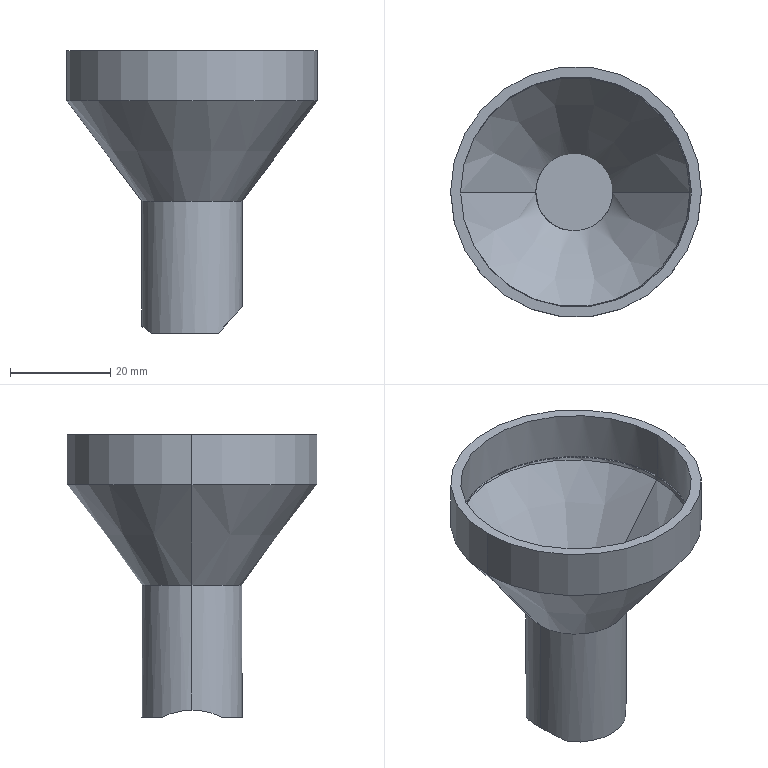Part | SolidWorks | features ICE 2, Blend 1, Cut 1, Extrusion 1, RefAxis 1, RevCut 1, SweepCut 1 | 1 solid | 21 faces | box 50 x 50 x 56.352 mm | volume 10137 mm3 | cylinder 8 | cone 6 | plane 5 | spline 2 | commonest cylinder face diameters 16 x2 20 x2 46 x2 50 x2
STEP:
#1=CARTESIAN_POINT('',(22.69,0.,-10.684));
#2=VERTEX_POINT('',#1);
#3=CARTESIAN_POINT('',(-23.,0.,-10.));
#4=VERTEX_POINT('',#3);
#5=CARTESIAN_POINT('',(-0.1549,0.,-10.342));
#6=DIRECTION('',(0.01498,0.,0.9999));
#7=DIRECTION('',(0.9999,0.,-0.01498));
#8=AXIS2_PLACEMENT_3D('',#5,#6,#7);
#9=CIRCLE('',#8,22.848);
#10=EDGE_CURVE('',#2,#4,#9,.T.);
#11=ORIENTED_EDGE('',*,*,#10,.F.);
#12=CARTESIAN_POINT('',(22.711,0.,-10.));
#13=VERTEX_POINT('',#12);
#14=CARTESIAN_POINT('',(22.69,0.,-10.684));
#15=DIRECTION('',(0.02995,0.,0.9996));
#16=VECTOR('',#15,1000.);
#17=LINE('',#14,#16);
#18=EDGE_CURVE('',#2,#13,#17,.T.);
#19=ORIENTED_EDGE('',*,*,#18,.T.);
#20=CARTESIAN_POINT('',(-23.,0.,-10.));
#21=CARTESIAN_POINT('',(-23.,45.706,-10.));
#22=CARTESIAN_POINT('',(22.711,45.706,-10.));
#23=CARTESIAN_POINT('',(22.711,0.,-10.));
#24=(BOUNDED_CURVE()B_SPLINE_CURVE(3,(#20,#21,#22,#23),.UNSPECIFIED.,.F.,.T.)B_SPLINE_CURVE_WITH_KNOTS((4,4),(3.142,6.283),.UNSPECIFIED.)CURVE()GEOMETRIC_REPRESENTATION_ITEM()RATIONAL_B_SPLINE_CURVE((1.,0.3333,0.3333,1.))REPRESENTATION_ITEM(''));
#25=EDGE_CURVE('',#4,#13,#24,.T.);
#26=ORIENTED_EDGE('',*,*,#25,.F.);
#27=EDGE_LOOP('',(#11,#19,#26));
#28=FACE_OUTER_BOUND('',#27,.T.);
#29=CARTESIAN_POINT('',(-0.1549,0.,-10.342));
#30=DIRECTION('',(0.01498,0.,0.9999));
#31=DIRECTION('',(0.9999,0.,-0.01498));
#32=AXIS2_PLACEMENT_3D('',#29,#30,#31);
#33=CONICAL_SURFACE('',#32,22.848,0.01498);
#34=ADVANCED_FACE('',(#28),#33,.F.);
#35=CARTESIAN_POINT('',(-8.,0.,-30.));
#36=VERTEX_POINT('',#35);
#37=CARTESIAN_POINT('',(7.278,0.,-30.));
#38=VERTEX_POINT('',#37);
#39=CARTESIAN_POINT('',(-8.,0.,-30.));
#40=CARTESIAN_POINT('',(-8.,-15.276,-30.));
#41=CARTESIAN_POINT('',(7.278,-15.276,-30.));
#42=CARTESIAN_POINT('',(7.278,0.,-30.));
#43=(BOUNDED_CURVE()B_SPLINE_CURVE(3,(#39,#40,#41,#42),.UNSPECIFIED.,.F.,.F.)B_SPLINE_CURVE_WITH_KNOTS((4,4),(3.142,6.283),.UNSPECIFIED.)CURVE()GEOMETRIC_REPRESENTATION_ITEM()RATIONAL_B_SPLINE_CURVE((1.,0.3333,0.3333,1.))REPRESENTATION_ITEM(''));
#44=EDGE_CURVE('',#36,#38,#43,.T.);
#45=ORIENTED_EDGE('',*,*,#44,.F.);
#46=CARTESIAN_POINT('',(-8.,0.,-30.));
#47=DIRECTION('',(-0.6,0.,0.8));
#48=VECTOR('',#47,1000.);
#49=LINE('',#46,#48);
#50=EDGE_CURVE('',#36,#4,#49,.T.);
#51=ORIENTED_EDGE('',*,*,#50,.T.);
#52=CARTESIAN_POINT('',(-0.1549,0.,-10.342));
#53=DIRECTION('',(0.01498,0.,0.9999));
#54=DIRECTION('',(0.9999,0.,-0.01498));
#55=AXIS2_PLACEMENT_3D('',#52,#53,#54);
#56=CIRCLE('',#55,22.848);
#57=EDGE_CURVE('',#4,#2,#56,.T.);
#58=ORIENTED_EDGE('',*,*,#57,.T.);
#59=CARTESIAN_POINT('',(7.098,0.,-30.226));
#60=DIRECTION('',(0.6237,0.,0.7817));
#61=VECTOR('',#60,1000.);
#62=LINE('',#59,#61);
#63=EDGE_CURVE('',#38,#2,#62,.T.);
#64=ORIENTED_EDGE('',*,*,#63,.F.);
#65=EDGE_LOOP('',(#45,#51,#58,#64));
#66=FACE_OUTER_BOUND('',#65,.T.);
#67=CARTESIAN_POINT('',(-0.4511,0.,-30.113));
#68=DIRECTION('',(0.01498,0.,0.9999));
#69=DIRECTION('',(0.9999,0.,-0.01498));
#70=AXIS2_PLACEMENT_3D('',#67,#68,#69);
#71=CONICAL_SURFACE('',#70,7.55,0.6585);
#72=ADVANCED_FACE('',(#66),#71,.F.);
#73=CARTESIAN_POINT('',(-8.,0.,-54.334));
#74=VERTEX_POINT('',#73);
#75=CARTESIAN_POINT('',(-3.42,-7.232,-56.352));
#76=VERTEX_POINT('',#75);
#77=CARTESIAN_POINT('',(-8.,0.,-54.334));
#78=CARTESIAN_POINT('',(-8.,-0.3871,-54.334));
#79=CARTESIAN_POINT('',(-7.971,-0.779,-54.35));
#80=CARTESIAN_POINT('',(-7.86,-1.541,-54.411));
#81=CARTESIAN_POINT('',(-7.777,-1.915,-54.456));
#82=CARTESIAN_POINT('',(-7.559,-2.648,-54.575));
#83=CARTESIAN_POINT('',(-7.422,-3.009,-54.648));
#84=CARTESIAN_POINT('',(-7.106,-3.695,-54.816));
#85=CARTESIAN_POINT('',(-6.925,-4.023,-54.91));
#86=CARTESIAN_POINT('',(-6.52,-4.65,-55.114));
#87=CARTESIAN_POINT('',(-6.295,-4.951,-55.226));
#88=CARTESIAN_POINT('',(-5.811,-5.511,-55.455));
#89=CARTESIAN_POINT('',(-5.552,-5.771,-55.573));
#90=CARTESIAN_POINT('',(-5.,-6.256,-55.81));
#91=CARTESIAN_POINT('',(-4.704,-6.481,-55.929));
#92=CARTESIAN_POINT('',(-4.082,-6.89,-56.154));
#93=CARTESIAN_POINT('',(-3.758,-7.072,-56.26));
#94=CARTESIAN_POINT('',(-3.42,-7.232,-56.352));
#95=B_SPLINE_CURVE_WITH_KNOTS('',3,(#77,#78,#79,#80,#81,#82,#83,#84,#85,#86,#87,#88,#89,#90,#91,#92,#93,#94),.UNSPECIFIED.,.F.,.F.,(4,2,2,2,2,2,2,2,4),(0.02654,0.02769,0.02885,0.03,0.03116,0.03231,0.03347,0.03462,0.03578),.UNSPECIFIED.);
#96=EDGE_CURVE('',#74,#76,#95,.T.);
#97=ORIENTED_EDGE('',*,*,#96,.F.);
#98=CARTESIAN_POINT('',(-8.,0.,-40.));
#99=DIRECTION('',(0.,0.,1.));
#100=VECTOR('',#99,1000.);
#101=LINE('',#98,#100);
#102=EDGE_CURVE('',#74,#36,#101,.T.);
#103=ORIENTED_EDGE('',*,*,#102,.T.);
#104=CARTESIAN_POINT('',(8.,0.,-30.));
#105=VERTEX_POINT('',#104);
#106=CARTESIAN_POINT('',(0.,0.,-30.));
#107=DIRECTION('',(0.,0.,1.));
#108=DIRECTION('',(-1.,0.,0.));
#109=AXIS2_PLACEMENT_3D('',#106,#107,#108);
#110=CIRCLE('',#109,8.);
#111=EDGE_CURVE('',#36,#105,#110,.T.);
#112=ORIENTED_EDGE('',*,*,#111,.T.);
#113=CARTESIAN_POINT('',(8.,0.,-51.21));
#114=VERTEX_POINT('',#113);
#115=CARTESIAN_POINT('',(8.,0.,-40.));
#116=DIRECTION('',(0.,0.,1.));
#117=VECTOR('',#116,1000.);
#118=LINE('',#115,#117);
#119=EDGE_CURVE('',#114,#105,#118,.T.);
#120=ORIENTED_EDGE('',*,*,#119,.F.);
#121=CARTESIAN_POINT('',(0.6884,-7.97,-56.352));
#122=VERTEX_POINT('',#121);
#123=CARTESIAN_POINT('',(0.6884,-7.97,-56.352));
#124=CARTESIAN_POINT('',(0.9487,-7.948,-56.271));
#125=CARTESIAN_POINT('',(1.206,-7.913,-56.175));
#126=CARTESIAN_POINT('',(1.702,-7.821,-55.964));
#127=CARTESIAN_POINT('',(1.942,-7.765,-55.848));
#128=CARTESIAN_POINT('',(2.408,-7.633,-55.603));
#129=CARTESIAN_POINT('',(2.635,-7.557,-55.473));
#130=CARTESIAN_POINT('',(3.079,-7.388,-55.203));
#131=CARTESIAN_POINT('',(3.296,-7.293,-55.063));
#132=CARTESIAN_POINT('',(3.926,-6.986,-54.637));
#133=CARTESIAN_POINT('',(4.318,-6.75,-54.347));
#134=CARTESIAN_POINT('',(5.061,-6.212,-53.771));
#135=CARTESIAN_POINT('',(5.412,-5.911,-53.486));
#136=CARTESIAN_POINT('',(6.072,-5.231,-52.932));
#137=CARTESIAN_POINT('',(6.374,-4.859,-52.671));
#138=CARTESIAN_POINT('',(6.781,-4.251,-52.312));
#139=CARTESIAN_POINT('',(6.909,-4.04,-52.199));
#140=CARTESIAN_POINT('',(7.15,-3.598,-51.984));
#141=CARTESIAN_POINT('',(7.262,-3.366,-51.883));
#142=CARTESIAN_POINT('',(7.564,-2.655,-51.61));
#143=CARTESIAN_POINT('',(7.723,-2.156,-51.465));
#144=CARTESIAN_POINT('',(7.888,-1.362,-51.313));
#145=CARTESIAN_POINT('',(7.93,-1.092,-51.275));
#146=CARTESIAN_POINT('',(7.986,-0.5495,-51.223));
#147=CARTESIAN_POINT('',(8.,-0.276,-51.21));
#148=CARTESIAN_POINT('',(8.,0.,-51.21));
#149=B_SPLINE_CURVE_WITH_KNOTS('',3,(#123,#124,#125,#126,#127,#128,#129,#130,#131,#132,#133,#134,#135,#136,#137,#138,#139,#140,#141,#142,#143,#144,#145,#146,#147,#148),.UNSPECIFIED.,.F.,.F.,(4,2,2,2,2,2,2,2,2,2,2,2,4),(0.04003,0.04084,0.04166,0.04247,0.04328,0.04491,0.04654,0.04817,0.04898,0.04979,0.05142,0.05224,0.05305),.UNSPECIFIED.);
#150=EDGE_CURVE('',#122,#114,#149,.T.);
#151=ORIENTED_EDGE('',*,*,#150,.F.);
#152=CARTESIAN_POINT('',(0.,0.,-56.352));
#153=DIRECTION('',(0.,0.,1.));
#154=DIRECTION('',(1.,0.,0.));
#155=AXIS2_PLACEMENT_3D('',#152,#153,#154);
#156=CIRCLE('',#155,8.);
#157=EDGE_CURVE('',#76,#122,#156,.T.);
#158=ORIENTED_EDGE('',*,*,#157,.F.);
#159=EDGE_LOOP('',(#97,#103,#112,#120,#151,#158));
#160=FACE_OUTER_BOUND('',#159,.T.);
#161=CARTESIAN_POINT('',(0.,0.,-40.));
#162=DIRECTION('',(0.,0.,1.));
#163=DIRECTION('',(1.,0.,0.));
#164=AXIS2_PLACEMENT_3D('',#161,#162,#163);
#165=CYLINDRICAL_SURFACE('',#164,8.);
#166=ADVANCED_FACE('',(#160),#165,.F.);
#167=CARTESIAN_POINT('',(-8.076,5.897,-56.352));
#168=VERTEX_POINT('',#167);
#169=CARTESIAN_POINT('',(-10.,0.,-54.908));
#170=VERTEX_POINT('',#169);
#171=CARTESIAN_POINT('',(-8.076,5.897,-56.352));
#172=CARTESIAN_POINT('',(-8.369,5.496,-56.131));
#173=CARTESIAN_POINT('',(-8.635,5.069,-55.93));
#174=CARTESIAN_POINT('',(-9.109,4.158,-55.574));
#175=CARTESIAN_POINT('',(-9.317,3.671,-55.418));
#176=CARTESIAN_POINT('',(-9.651,2.671,-55.168));
#177=CARTESIAN_POINT('',(-9.78,2.154,-55.072));
#178=CARTESIAN_POINT('',(-9.912,1.351,-54.973));
#179=CARTESIAN_POINT('',(-9.945,1.079,-54.949));
#180=CARTESIAN_POINT('',(-9.989,0.5395,-54.916));
#181=CARTESIAN_POINT('',(-10.,0.2697,-54.908));
#182=CARTESIAN_POINT('',(-10.,0.,-54.908));
#183=B_SPLINE_CURVE_WITH_KNOTS('',3,(#171,#172,#173,#174,#175,#176,#177,#178,#179,#180,#181,#182),.UNSPECIFIED.,.F.,.F.,(4,2,2,2,2,4),(0.01131,0.01294,0.01457,0.01619,0.01701,0.01782),.UNSPECIFIED.);
#184=EDGE_CURVE('',#168,#170,#183,.T.);
#185=ORIENTED_EDGE('',*,*,#184,.T.);
#186=CARTESIAN_POINT('',(-10.,0.,-30.));
#187=VERTEX_POINT('',#186);
#188=CARTESIAN_POINT('',(-10.,0.,-40.));
#189=DIRECTION('',(0.,0.,1.));
#190=VECTOR('',#189,1000.);
#191=LINE('',#188,#190);
#192=EDGE_CURVE('',#170,#187,#191,.T.);
#193=ORIENTED_EDGE('',*,*,#192,.T.);
#194=CARTESIAN_POINT('',(10.,0.,-30.));
#195=VERTEX_POINT('',#194);
#196=CARTESIAN_POINT('',(0.,0.,-30.));
#197=DIRECTION('',(0.,0.,-1.));
#198=DIRECTION('',(-1.,0.,0.));
#199=AXIS2_PLACEMENT_3D('',#196,#197,#198);
#200=CIRCLE('',#199,10.);
#201=EDGE_CURVE('',#187,#195,#200,.T.);
#202=ORIENTED_EDGE('',*,*,#201,.T.);
#203=CARTESIAN_POINT('',(10.,0.,-50.997));
#204=VERTEX_POINT('',#203);
#205=CARTESIAN_POINT('',(10.,0.,-40.));
#206=DIRECTION('',(0.,0.,1.));
#207=VECTOR('',#206,1000.);
#208=LINE('',#205,#207);
#209=EDGE_CURVE('',#204,#195,#208,.T.);
#210=ORIENTED_EDGE('',*,*,#209,.F.);
#211=CARTESIAN_POINT('',(5.262,8.504,-56.352));
#212=VERTEX_POINT('',#211);
#213=CARTESIAN_POINT('',(10.,0.,-50.997));
#214=CARTESIAN_POINT('',(10.,0.4979,-50.997));
#215=CARTESIAN_POINT('',(9.963,0.9852,-51.037));
#216=CARTESIAN_POINT('',(9.857,1.702,-51.154));
#217=CARTESIAN_POINT('',(9.813,1.938,-51.203));
#218=CARTESIAN_POINT('',(9.709,2.406,-51.318));
#219=CARTESIAN_POINT('',(9.648,2.639,-51.385));
#220=CARTESIAN_POINT('',(9.446,3.316,-51.609));
#221=CARTESIAN_POINT('',(9.284,3.743,-51.788));
#222=CARTESIAN_POINT('',(8.913,4.556,-52.201));
#223=CARTESIAN_POINT('',(8.703,4.943,-52.435));
#224=CARTESIAN_POINT('',(8.031,6.018,-53.187));
#225=CARTESIAN_POINT('',(7.524,6.631,-53.758));
#226=CARTESIAN_POINT('',(6.426,7.7,-55.009));
#227=CARTESIAN_POINT('',(5.852,8.138,-55.667));
#228=CARTESIAN_POINT('',(5.262,8.504,-56.352));
#229=B_SPLINE_CURVE_WITH_KNOTS('',3,(#213,#214,#215,#216,#217,#218,#219,#220,#221,#222,#223,#224,#225,#226,#227,#228),.UNSPECIFIED.,.F.,.F.,(4,2,2,2,2,2,2,4),(0.01995,0.0214,0.02213,0.02286,0.02431,0.02577,0.02868,0.03159),.UNSPECIFIED.);
#230=EDGE_CURVE('',#204,#212,#229,.T.);
#231=ORIENTED_EDGE('',*,*,#230,.T.);
#232=CARTESIAN_POINT('',(0.,0.,-56.352));
#233=DIRECTION('',(0.,0.,1.));
#234=DIRECTION('',(1.,0.,0.));
#235=AXIS2_PLACEMENT_3D('',#232,#233,#234);
#236=CIRCLE('',#235,10.);
#237=EDGE_CURVE('',#212,#168,#236,.T.);
#238=ORIENTED_EDGE('',*,*,#237,.T.);
#239=EDGE_LOOP('',(#185,#193,#202,#210,#231,#238));
#240=FACE_OUTER_BOUND('',#239,.T.);
#241=CARTESIAN_POINT('',(0.,0.,-40.));
#242=DIRECTION('',(0.,0.,1.));
#243=DIRECTION('',(1.,0.,0.));
#244=AXIS2_PLACEMENT_3D('',#241,#242,#243);
#245=CYLINDRICAL_SURFACE('',#244,10.);
#246=ADVANCED_FACE('',(#240),#245,.T.);
#247=ORIENTED_EDGE('',*,*,#201,.F.);
#248=CARTESIAN_POINT('',(-25.,0.,-10.));
#249=VERTEX_POINT('',#248);
#250=CARTESIAN_POINT('',(-10.,0.,-30.));
#251=DIRECTION('',(-0.6,0.,0.8));
#252=VECTOR('',#251,1000.);
#253=LINE('',#250,#252);
#254=EDGE_CURVE('',#187,#249,#253,.T.);
#255=ORIENTED_EDGE('',*,*,#254,.T.);
#256=CARTESIAN_POINT('',(25.,0.,-10.));
#257=VERTEX_POINT('',#256);
#258=CARTESIAN_POINT('',(0.,0.,-10.));
#259=DIRECTION('',(0.,0.,1.));
#260=DIRECTION('',(1.,0.,0.));
#261=AXIS2_PLACEMENT_3D('',#258,#259,#260);
#262=CIRCLE('',#261,25.);
#263=EDGE_CURVE('',#257,#249,#262,.T.);
#264=ORIENTED_EDGE('',*,*,#263,.F.);
#265=CARTESIAN_POINT('',(10.,0.,-30.));
#266=DIRECTION('',(0.6,0.,0.8));
#267=VECTOR('',#266,1000.);
#268=LINE('',#265,#267);
#269=EDGE_CURVE('',#195,#257,#268,.T.);
#270=ORIENTED_EDGE('',*,*,#269,.F.);
#271=EDGE_LOOP('',(#247,#255,#264,#270));
#272=FACE_OUTER_BOUND('',#271,.T.);
#273=CARTESIAN_POINT('',(0.,0.,-30.));
#274=DIRECTION('',(0.,0.,1.));
#275=DIRECTION('',(1.,0.,0.));
#276=AXIS2_PLACEMENT_3D('',#273,#274,#275);
#277=CONICAL_SURFACE('',#276,10.,0.6435);
#278=ADVANCED_FACE('',(#272),#277,.T.);
#279=CARTESIAN_POINT('',(23.,0.,-10.));
#280=VERTEX_POINT('',#279);
#281=CARTESIAN_POINT('',(0.,0.,-10.));
#282=DIRECTION('',(0.,0.,1.));
#283=DIRECTION('',(1.,0.,0.));
#284=AXIS2_PLACEMENT_3D('',#281,#282,#283);
#285=CIRCLE('',#284,23.);
#286=EDGE_CURVE('',#4,#280,#285,.T.);
#287=ORIENTED_EDGE('',*,*,#286,.F.);
#288=CARTESIAN_POINT('',(-23.,0.,0.));
#289=VERTEX_POINT('',#288);
#290=CARTESIAN_POINT('',(-23.,0.,-10.));
#291=DIRECTION('',(0.,0.,1.));
#292=VECTOR('',#291,1000.);
#293=LINE('',#290,#292);
#294=EDGE_CURVE('',#4,#289,#293,.T.);
#295=ORIENTED_EDGE('',*,*,#294,.T.);
#296=CARTESIAN_POINT('',(23.,0.,0.));
#297=VERTEX_POINT('',#296);
#298=CARTESIAN_POINT('',(0.,0.,0.));
#299=DIRECTION('',(0.,0.,1.));
#300=DIRECTION('',(1.,0.,0.));
#301=AXIS2_PLACEMENT_3D('',#298,#299,#300);
#302=CIRCLE('',#301,23.);
#303=EDGE_CURVE('',#289,#297,#302,.T.);
#304=ORIENTED_EDGE('',*,*,#303,.T.);
#305=CARTESIAN_POINT('',(23.,0.,-10.));
#306=DIRECTION('',(0.,0.,1.));
#307=VECTOR('',#306,1000.);
#308=LINE('',#305,#307);
#309=EDGE_CURVE('',#280,#297,#308,.T.);
#310=ORIENTED_EDGE('',*,*,#309,.F.);
#311=EDGE_LOOP('',(#287,#295,#304,#310));
#312=FACE_OUTER_BOUND('',#311,.T.);
#313=CARTESIAN_POINT('',(0.,0.,-10.));
#314=DIRECTION('',(0.,0.,1.));
#315=DIRECTION('',(1.,0.,0.));
#316=AXIS2_PLACEMENT_3D('',#313,#314,#315);
#317=CYLINDRICAL_SURFACE('',#316,23.);
#318=ADVANCED_FACE('',(#312),#317,.F.);
#319=ORIENTED_EDGE('',*,*,#263,.T.);
#320=CARTESIAN_POINT('',(-25.,0.,0.));
#321=VERTEX_POINT('',#320);
#322=CARTESIAN_POINT('',(-25.,0.,-10.));
#323=DIRECTION('',(0.,0.,1.));
#324=VECTOR('',#323,1000.);
#325=LINE('',#322,#324);
#326=EDGE_CURVE('',#249,#321,#325,.T.);
#327=ORIENTED_EDGE('',*,*,#326,.T.);
#328=CARTESIAN_POINT('',(25.,0.,0.));
#329=VERTEX_POINT('',#328);
#330=CARTESIAN_POINT('',(0.,0.,0.));
#331=DIRECTION('',(0.,0.,1.));
#332=DIRECTION('',(1.,0.,0.));
#333=AXIS2_PLACEMENT_3D('',#330,#331,#332);
#334=CIRCLE('',#333,25.);
#335=EDGE_CURVE('',#329,#321,#334,.T.);
#336=ORIENTED_EDGE('',*,*,#335,.F.);
#337=CARTESIAN_POINT('',(25.,0.,-10.));
#338=DIRECTION('',(0.,0.,1.));
#339=VECTOR('',#338,1000.);
#340=LINE('',#337,#339);
#341=EDGE_CURVE('',#257,#329,#340,.T.);
#342=ORIENTED_EDGE('',*,*,#341,.F.);
#343=EDGE_LOOP('',(#319,#327,#336,#342));
#344=FACE_OUTER_BOUND('',#343,.T.);
#345=CARTESIAN_POINT('',(0.,0.,-10.));
#346=DIRECTION('',(0.,0.,1.));
#347=DIRECTION('',(1.,0.,0.));
#348=AXIS2_PLACEMENT_3D('',#345,#346,#347);
#349=CYLINDRICAL_SURFACE('',#348,25.);
#350=ADVANCED_FACE('',(#344),#349,.T.);
#351=ORIENTED_EDGE('',*,*,#184,.F.);
#352=CARTESIAN_POINT('',(-3.42,7.232,-56.352));
#353=VERTEX_POINT('',#352);
#354=CARTESIAN_POINT('',(-8.076,5.897,-56.352));
#355=CARTESIAN_POINT('',(-7.315,6.181,-56.352));
#356=CARTESIAN_POINT('',(-6.545,6.427,-56.352));
#357=CARTESIAN_POINT('',(-4.992,6.866,-56.352));
#358=CARTESIAN_POINT('',(-4.208,7.059,-56.352));
#359=CARTESIAN_POINT('',(-3.42,7.232,-56.352));
#360=B_SPLINE_CURVE_WITH_KNOTS('',3,(#354,#355,#356,#357,#358,#359),.UNSPECIFIED.,.F.,.F.,(4,2,4),(0.001732,0.004153,0.006575),.UNSPECIFIED.);
#361=EDGE_CURVE('',#168,#353,#360,.T.);
#362=ORIENTED_EDGE('',*,*,#361,.T.);
#363=CARTESIAN_POINT('',(-3.42,7.232,-56.352));
#364=CARTESIAN_POINT('',(-3.759,7.072,-56.26));
#365=CARTESIAN_POINT('',(-4.083,6.89,-56.154));
#366=CARTESIAN_POINT('',(-4.705,6.481,-55.928));
#367=CARTESIAN_POINT('',(-5.002,6.254,-55.809));
#368=CARTESIAN_POINT('',(-5.556,5.768,-55.571));
#369=CARTESIAN_POINT('',(-5.816,5.506,-55.453));
#370=CARTESIAN_POINT('',(-6.3,4.945,-55.224));
#371=CARTESIAN_POINT('',(-6.526,4.643,-55.112));
#372=CARTESIAN_POINT('',(-7.132,3.701,-54.805));
#373=CARTESIAN_POINT('',(-7.448,3.021,-54.635));
#374=CARTESIAN_POINT('',(-7.778,1.91,-54.456));
#375=CARTESIAN_POINT('',(-7.861,1.532,-54.41));
#376=CARTESIAN_POINT('',(-7.972,0.7722,-54.349));
#377=CARTESIAN_POINT('',(-8.,0.3881,-54.334));
#378=CARTESIAN_POINT('',(-8.,0.,-54.334));
#379=B_SPLINE_CURVE_WITH_KNOTS('',3,(#363,#364,#365,#366,#367,#368,#369,#370,#371,#372,#373,#374,#375,#376,#377,#378),.UNSPECIFIED.,.F.,.F.,(4,2,2,2,2,2,2,4),(0.01727,0.01843,0.01959,0.02075,0.02191,0.02422,0.02538,0.02654),.UNSPECIFIED.);
#380=EDGE_CURVE('',#353,#74,#379,.T.);
#381=ORIENTED_EDGE('',*,*,#380,.T.);
#382=ORIENTED_EDGE('',*,*,#96,.T.);
#383=CARTESIAN_POINT('',(-8.076,-5.897,-56.352));
#384=VERTEX_POINT('',#383);
#385=CARTESIAN_POINT('',(-3.42,-7.232,-56.352));
#386=CARTESIAN_POINT('',(-4.205,-7.06,-56.352));
#387=CARTESIAN_POINT('',(-4.986,-6.867,-56.352));
#388=CARTESIAN_POINT('',(-6.539,-6.429,-56.352));
#389=CARTESIAN_POINT('',(-7.311,-6.183,-56.352));
#390=CARTESIAN_POINT('',(-8.076,-5.897,-56.352));
#391=B_SPLINE_CURVE_WITH_KNOTS('',3,(#385,#386,#387,#388,#389,#390),.UNSPECIFIED.,.F.,.F.,(4,2,4),(0.01423,0.01664,0.01905),.UNSPECIFIED.);
#392=EDGE_CURVE('',#76,#384,#391,.T.);
#393=ORIENTED_EDGE('',*,*,#392,.T.);
#394=CARTESIAN_POINT('',(-10.,0.,-54.908));
#395=CARTESIAN_POINT('',(-10.,-0.5412,-54.908));
#396=CARTESIAN_POINT('',(-9.956,-1.084,-54.941));
#397=CARTESIAN_POINT('',(-9.779,-2.16,-55.073));
#398=CARTESIAN_POINT('',(-9.649,-2.677,-55.169));
#399=CARTESIAN_POINT('',(-9.317,-3.671,-55.418));
#400=CARTESIAN_POINT('',(-9.113,-4.149,-55.571));
#401=CARTESIAN_POINT('',(-8.756,-4.838,-55.84));
#402=CARTESIAN_POINT('',(-8.628,-5.061,-55.936));
#403=CARTESIAN_POINT('',(-8.362,-5.491,-56.137));
#404=CARTESIAN_POINT('',(-8.222,-5.698,-56.242));
#405=CARTESIAN_POINT('',(-8.076,-5.897,-56.352));
#406=B_SPLINE_CURVE_WITH_KNOTS('',3,(#394,#395,#396,#397,#398,#399,#400,#401,#402,#403,#404,#405),.UNSPECIFIED.,.F.,.F.,(4,2,2,2,2,4),(0.01782,0.01946,0.02109,0.02272,0.02354,0.02436),.UNSPECIFIED.);
#407=EDGE_CURVE('',#170,#384,#406,.T.);
#408=ORIENTED_EDGE('',*,*,#407,.F.);
#409=EDGE_LOOP('',(#351,#362,#381,#382,#393,#408));
#410=FACE_OUTER_BOUND('',#409,.T.);
#411=CARTESIAN_POINT('',(100.251,0.,-188.146));
#412=CARTESIAN_POINT('',(36.995,0.,-348.142));
#413=CARTESIAN_POINT('',(-123.001,0.,-284.887));
#414=CARTESIAN_POINT('',(-59.745,0.,-124.891));
#415=CARTESIAN_POINT('',(3.511,0.,35.105));
#416=CARTESIAN_POINT('',(163.507,0.,-28.151));
#417=CARTESIAN_POINT('',(100.251,0.,-188.146));
#418=CARTESIAN_POINT('',(100.251,20.,-188.146));
#419=CARTESIAN_POINT('',(36.995,20.,-348.142));
#420=CARTESIAN_POINT('',(-123.001,20.,-284.887));
#421=CARTESIAN_POINT('',(-59.745,20.,-124.891));
#422=CARTESIAN_POINT('',(3.511,20.,35.105));
#423=CARTESIAN_POINT('',(163.507,20.,-28.151));
#424=CARTESIAN_POINT('',(100.251,20.,-188.146));
#425=CARTESIAN_POINT('',(119.016,20.,-195.065));
#426=CARTESIAN_POINT('',(41.922,20.,-392.591));
#427=CARTESIAN_POINT('',(-155.604,20.,-315.498));
#428=CARTESIAN_POINT('',(-78.51,20.,-117.972));
#429=CARTESIAN_POINT('',(-1.416,20.,79.554));
#430=CARTESIAN_POINT('',(196.11,20.,2.461));
#431=CARTESIAN_POINT('',(119.016,20.,-195.065));
#432=CARTESIAN_POINT('',(119.016,0.,-195.065));
#433=CARTESIAN_POINT('',(41.922,0.,-392.591));
#434=CARTESIAN_POINT('',(-155.604,0.,-315.498));
#435=CARTESIAN_POINT('',(-78.51,0.,-117.972));
#436=CARTESIAN_POINT('',(-1.416,0.,79.554));
#437=CARTESIAN_POINT('',(196.11,0.,2.461));
#438=CARTESIAN_POINT('',(119.016,0.,-195.065));
#439=CARTESIAN_POINT('',(119.016,-20.,-195.065));
#440=CARTESIAN_POINT('',(41.922,-20.,-392.591));
#441=CARTESIAN_POINT('',(-155.604,-20.,-315.498));
#442=CARTESIAN_POINT('',(-78.51,-20.,-117.972));
#443=CARTESIAN_POINT('',(-1.416,-20.,79.554));
#444=CARTESIAN_POINT('',(196.11,-20.,2.461));
#445=CARTESIAN_POINT('',(119.016,-20.,-195.065));
#446=CARTESIAN_POINT('',(100.251,-20.,-188.146));
#447=CARTESIAN_POINT('',(36.995,-20.,-348.142));
#448=CARTESIAN_POINT('',(-123.001,-20.,-284.887));
#449=CARTESIAN_POINT('',(-59.745,-20.,-124.891));
#450=CARTESIAN_POINT('',(3.511,-20.,35.105));
#451=CARTESIAN_POINT('',(163.507,-20.,-28.151));
#452=CARTESIAN_POINT('',(100.251,-20.,-188.146));
#453=CARTESIAN_POINT('',(100.251,0.,-188.146));
#454=CARTESIAN_POINT('',(36.995,0.,-348.142));
#455=CARTESIAN_POINT('',(-123.001,0.,-284.887));
#456=CARTESIAN_POINT('',(-59.745,0.,-124.891));
#457=CARTESIAN_POINT('',(3.511,0.,35.105));
#458=CARTESIAN_POINT('',(163.507,0.,-28.151));
#459=CARTESIAN_POINT('',(100.251,0.,-188.146));
#460=(BOUNDED_SURFACE()B_SPLINE_SURFACE(3,3,((#411,#412,#413,#414,#415,#416,#417),(#418,#419,#420,#421,#422,#423,#424),(#425,#426,#427,#428,#429,#430,#431),(#432,#433,#434,#435,#436,#437,#438),(#439,#440,#441,#442,#443,#444,#445),(#446,#447,#448,#449,#450,#451,#452),(#453,#454,#455,#456,#457,#458,#459)),.UNSPECIFIED.,.T.,.T.,.F.)B_SPLINE_SURFACE_WITH_KNOTS((4,3,4),(4,3,4),(0.,0.5,1.),(0.,0.5,1.),.UNSPECIFIED.)GEOMETRIC_REPRESENTATION_ITEM()RATIONAL_B_SPLINE_SURFACE(((1.,0.3333,0.3333,1.,0.3333,0.3333,1.),(0.3333,0.1111,0.1111,0.3333,0.1111,0.1111,0.3333),(0.3333,0.1111,0.1111,0.3333,0.1111,0.1111,0.3333),(1.,0.3333,0.3333,1.,0.3333,0.3333,1.),(0.3333,0.1111,0.1111,0.3333,0.1111,0.1111,0.3333),(0.3333,0.1111,0.1111,0.3333,0.1111,0.1111,0.3333),(1.,0.3333,0.3333,1.,0.3333,0.3333,1.)))REPRESENTATION_ITEM('')SURFACE());
#461=ADVANCED_FACE('',(#410),#460,.F.);
#462=ORIENTED_EDGE('',*,*,#326,.F.);
#463=CARTESIAN_POINT('',(0.,0.,-10.));
#464=DIRECTION('',(0.,0.,1.));
#465=DIRECTION('',(1.,0.,0.));
#466=AXIS2_PLACEMENT_3D('',#463,#464,#465);
#467=CIRCLE('',#466,25.);
#468=EDGE_CURVE('',#249,#257,#467,.T.);
#469=ORIENTED_EDGE('',*,*,#468,.T.);
#470=ORIENTED_EDGE('',*,*,#341,.T.);
#471=CARTESIAN_POINT('',(0.,0.,0.));
#472=DIRECTION('',(0.,0.,1.));
#473=DIRECTION('',(1.,0.,0.));
#474=AXIS2_PLACEMENT_3D('',#471,#472,#473);
#475=CIRCLE('',#474,25.);
#476=EDGE_CURVE('',#321,#329,#475,.T.);
#477=ORIENTED_EDGE('',*,*,#476,.F.);
#478=EDGE_LOOP('',(#462,#469,#470,#477));
#479=FACE_OUTER_BOUND('',#478,.T.);
#480=CARTESIAN_POINT('',(0.,0.,-10.));
#481=DIRECTION('',(0.,0.,1.));
#482=DIRECTION('',(1.,0.,0.));
#483=AXIS2_PLACEMENT_3D('',#480,#481,#482);
#484=CYLINDRICAL_SURFACE('',#483,25.);
#485=ADVANCED_FACE('',(#479),#484,.T.);
#486=CARTESIAN_POINT('',(0.,0.,0.));
#487=DIRECTION('',(0.,0.,1.));
#488=DIRECTION('',(1.,0.,0.));
#489=AXIS2_PLACEMENT_3D('',#486,#487,#488);
#490=CIRCLE('',#489,23.);
#491=EDGE_CURVE('',#297,#289,#490,.T.);
#492=ORIENTED_EDGE('',*,*,#491,.F.);
#493=ORIENTED_EDGE('',*,*,#303,.F.);
#494=EDGE_LOOP('',(#492,#493));
#495=FACE_BOUND('',#494,.T.);
#496=ORIENTED_EDGE('',*,*,#335,.T.);
#497=ORIENTED_EDGE('',*,*,#476,.T.);
#498=EDGE_LOOP('',(#496,#497));
#499=FACE_OUTER_BOUND('',#498,.T.);
#500=CARTESIAN_POINT('',(0.,0.,0.));
#501=DIRECTION('',(0.,0.,1.));
#502=DIRECTION('',(1.,0.,0.));
#503=AXIS2_PLACEMENT_3D('',#500,#501,#502);
#504=PLANE('',#503);
#505=ADVANCED_FACE('',(#495,#499),#504,.T.);
#506=ORIENTED_EDGE('',*,*,#294,.F.);
#507=CARTESIAN_POINT('',(0.,0.,-10.));
#508=DIRECTION('',(0.,0.,1.));
#509=DIRECTION('',(1.,0.,0.));
#510=AXIS2_PLACEMENT_3D('',#507,#508,#509);
#511=CIRCLE('',#510,23.);
#512=EDGE_CURVE('',#280,#4,#511,.T.);
#513=ORIENTED_EDGE('',*,*,#512,.F.);
#514=ORIENTED_EDGE('',*,*,#309,.T.);
#515=ORIENTED_EDGE('',*,*,#491,.T.);
#516=EDGE_LOOP('',(#506,#513,#514,#515));
#517=FACE_OUTER_BOUND('',#516,.T.);
#518=CARTESIAN_POINT('',(0.,0.,-10.));
#519=DIRECTION('',(0.,0.,1.));
#520=DIRECTION('',(1.,0.,0.));
#521=AXIS2_PLACEMENT_3D('',#518,#519,#520);
#522=CYLINDRICAL_SURFACE('',#521,23.);
#523=ADVANCED_FACE('',(#517),#522,.F.);
#524=ORIENTED_EDGE('',*,*,#286,.T.);
#525=ORIENTED_EDGE('',*,*,#512,.T.);
#526=ORIENTED_EDGE('',*,*,#25,.T.);
#527=CARTESIAN_POINT('',(22.711,0.,-10.));
#528=CARTESIAN_POINT('',(22.711,-45.706,-10.));
#529=CARTESIAN_POINT('',(-23.,-45.706,-10.));
#530=CARTESIAN_POINT('',(-23.,0.,-10.));
#531=(BOUNDED_CURVE()B_SPLINE_CURVE(3,(#527,#528,#529,#530),.UNSPECIFIED.,.F.,.F.)B_SPLINE_CURVE_WITH_KNOTS((4,4),(0.,3.142),.UNSPECIFIED.)CURVE()GEOMETRIC_REPRESENTATION_ITEM()RATIONAL_B_SPLINE_CURVE((1.,0.3333,0.3333,1.))REPRESENTATION_ITEM(''));
#532=EDGE_CURVE('',#13,#4,#531,.T.);
#533=ORIENTED_EDGE('',*,*,#532,.T.);
#534=EDGE_LOOP('',(#524,#525,#526,#533));
#535=FACE_OUTER_BOUND('',#534,.T.);
#536=CARTESIAN_POINT('',(0.,0.,-10.));
#537=DIRECTION('',(0.,0.,1.));
#538=DIRECTION('',(1.,0.,0.));
#539=AXIS2_PLACEMENT_3D('',#536,#537,#538);
#540=PLANE('',#539);
#541=ADVANCED_FACE('',(#535),#540,.T.);
#542=ORIENTED_EDGE('',*,*,#254,.F.);
#543=CARTESIAN_POINT('',(0.,0.,-30.));
#544=DIRECTION('',(0.,0.,-1.));
#545=DIRECTION('',(-1.,0.,0.));
#546=AXIS2_PLACEMENT_3D('',#543,#544,#545);
#547=CIRCLE('',#546,10.);
#548=EDGE_CURVE('',#195,#187,#547,.T.);
#549=ORIENTED_EDGE('',*,*,#548,.F.);
#550=ORIENTED_EDGE('',*,*,#269,.T.);
#551=ORIENTED_EDGE('',*,*,#468,.F.);
#552=EDGE_LOOP('',(#542,#549,#550,#551));
#553=FACE_OUTER_BOUND('',#552,.T.);
#554=CARTESIAN_POINT('',(0.,0.,-30.));
#555=DIRECTION('',(0.,0.,1.));
#556=DIRECTION('',(1.,0.,0.));
#557=AXIS2_PLACEMENT_3D('',#554,#555,#556);
#558=CONICAL_SURFACE('',#557,10.,0.6435);
#559=ADVANCED_FACE('',(#553),#558,.T.);
#560=ORIENTED_EDGE('',*,*,#192,.F.);
#561=ORIENTED_EDGE('',*,*,#407,.T.);
#562=CARTESIAN_POINT('',(5.262,-8.504,-56.352));
#563=VERTEX_POINT('',#562);
#564=CARTESIAN_POINT('',(0.,0.,-56.352));
#565=DIRECTION('',(0.,0.,1.));
#566=DIRECTION('',(1.,0.,0.));
#567=AXIS2_PLACEMENT_3D('',#564,#565,#566);
#568=CIRCLE('',#567,10.);
#569=EDGE_CURVE('',#384,#563,#568,.T.);
#570=ORIENTED_EDGE('',*,*,#569,.T.);
#571=CARTESIAN_POINT('',(5.262,-8.504,-56.352));
#572=CARTESIAN_POINT('',(5.857,-8.135,-55.662));
#573=CARTESIAN_POINT('',(6.431,-7.696,-55.003));
#574=CARTESIAN_POINT('',(7.247,-6.901,-54.074));
#575=CARTESIAN_POINT('',(7.514,-6.611,-53.772));
#576=CARTESIAN_POINT('',(8.018,-5.989,-53.202));
#577=CARTESIAN_POINT('',(8.257,-5.656,-52.934));
#578=CARTESIAN_POINT('',(8.703,-4.943,-52.435));
#579=CARTESIAN_POINT('',(8.91,-4.562,-52.204));
#580=CARTESIAN_POINT('',(9.284,-3.744,-51.789));
#581=CARTESIAN_POINT('',(9.445,-3.317,-51.609));
#582=CARTESIAN_POINT('',(9.646,-2.646,-51.387));
#583=CARTESIAN_POINT('',(9.706,-2.417,-51.321));
#584=CARTESIAN_POINT('',(9.811,-1.949,-51.205));
#585=CARTESIAN_POINT('',(9.856,-1.709,-51.155));
#586=CARTESIAN_POINT('',(9.963,-0.9861,-51.037));
#587=CARTESIAN_POINT('',(10.,-0.497,-50.997));
#588=CARTESIAN_POINT('',(10.,0.,-50.997));
#589=B_SPLINE_CURVE_WITH_KNOTS('',3,(#571,#572,#573,#574,#575,#576,#577,#578,#579,#580,#581,#582,#583,#584,#585,#586,#587,#588),.UNSPECIFIED.,.F.,.F.,(4,2,2,2,2,2,2,2,4),(0.008329,0.01123,0.01269,0.01414,0.01559,0.01704,0.01777,0.0185,0.01995),.UNSPECIFIED.);
#590=EDGE_CURVE('',#563,#204,#589,.T.);
#591=ORIENTED_EDGE('',*,*,#590,.T.);
#592=ORIENTED_EDGE('',*,*,#209,.T.);
#593=ORIENTED_EDGE('',*,*,#548,.T.);
#594=EDGE_LOOP('',(#560,#561,#570,#591,#592,#593));
#595=FACE_OUTER_BOUND('',#594,.T.);
#596=CARTESIAN_POINT('',(0.,0.,-40.));
#597=DIRECTION('',(0.,0.,1.));
#598=DIRECTION('',(1.,0.,0.));
#599=AXIS2_PLACEMENT_3D('',#596,#597,#598);
#600=CYLINDRICAL_SURFACE('',#599,10.);
#601=ADVANCED_FACE('',(#595),#600,.T.);
#602=ORIENTED_EDGE('',*,*,#150,.T.);
#603=CARTESIAN_POINT('',(0.6884,7.97,-56.352));
#604=VERTEX_POINT('',#603);
#605=CARTESIAN_POINT('',(8.,0.,-51.21));
#606=CARTESIAN_POINT('',(8.,0.552,-51.21));
#607=CARTESIAN_POINT('',(7.944,1.09,-51.262));
#608=CARTESIAN_POINT('',(7.781,1.877,-51.411));
#609=CARTESIAN_POINT('',(7.714,2.137,-51.473));
#610=CARTESIAN_POINT('',(7.556,2.642,-51.617));
#611=CARTESIAN_POINT('',(7.466,2.887,-51.699));
#612=CARTESIAN_POINT('',(7.265,3.359,-51.88));
#613=CARTESIAN_POINT('',(7.155,3.588,-51.98));
#614=CARTESIAN_POINT('',(6.915,4.031,-52.194));
#615=CARTESIAN_POINT('',(6.785,4.246,-52.309));
#616=CARTESIAN_POINT('',(6.376,4.857,-52.669));
#617=CARTESIAN_POINT('',(6.075,5.226,-52.929));
#618=CARTESIAN_POINT('',(5.422,5.901,-53.477));
#619=CARTESIAN_POINT('',(5.067,6.208,-53.767));
#620=CARTESIAN_POINT('',(4.319,6.75,-54.346));
#621=CARTESIAN_POINT('',(3.926,6.986,-54.637));
#622=CARTESIAN_POINT('',(3.09,7.394,-55.202));
#623=CARTESIAN_POINT('',(2.643,7.566,-55.479));
#624=CARTESIAN_POINT('',(1.941,7.765,-55.848));
#625=CARTESIAN_POINT('',(1.701,7.821,-55.964));
#626=CARTESIAN_POINT('',(1.206,7.913,-56.175));
#627=CARTESIAN_POINT('',(0.9494,7.948,-56.271));
#628=CARTESIAN_POINT('',(0.6884,7.97,-56.352));
#629=B_SPLINE_CURVE_WITH_KNOTS('',3,(#605,#606,#607,#608,#609,#610,#611,#612,#613,#614,#615,#616,#617,#618,#619,#620,#621,#622,#623,#624,#625,#626,#627,#628),.UNSPECIFIED.,.F.,.F.,(4,2,2,2,2,2,2,2,2,2,2,4),(0.,0.001628,0.002442,0.003256,0.00407,0.004884,0.006511,0.008139,0.009767,0.0114,0.01221,0.01302),.UNSPECIFIED.);
#630=EDGE_CURVE('',#114,#604,#629,.T.);
#631=ORIENTED_EDGE('',*,*,#630,.T.);
#632=CARTESIAN_POINT('',(0.6884,7.97,-56.352));
#633=CARTESIAN_POINT('',(2.207,8.191,-56.352));
#634=CARTESIAN_POINT('',(3.734,8.364,-56.352));
#635=CARTESIAN_POINT('',(5.262,8.504,-56.352));
#636=B_SPLINE_CURVE_WITH_KNOTS('',3,(#632,#633,#634,#635),.UNSPECIFIED.,.F.,.F.,(4,4),(0.01074,0.01531),.UNSPECIFIED.);
#637=EDGE_CURVE('',#604,#212,#636,.T.);
#638=ORIENTED_EDGE('',*,*,#637,.T.);
#639=ORIENTED_EDGE('',*,*,#230,.F.);
#640=ORIENTED_EDGE('',*,*,#590,.F.);
#641=CARTESIAN_POINT('',(5.262,-8.504,-56.352));
#642=CARTESIAN_POINT('',(3.731,-8.363,-56.352));
#643=CARTESIAN_POINT('',(2.205,-8.191,-56.352));
#644=CARTESIAN_POINT('',(0.6884,-7.97,-56.352));
#645=B_SPLINE_CURVE_WITH_KNOTS('',3,(#641,#642,#643,#644),.UNSPECIFIED.,.F.,.F.,(4,4),(0.005462,0.01006),.UNSPECIFIED.);
#646=EDGE_CURVE('',#563,#122,#645,.T.);
#647=ORIENTED_EDGE('',*,*,#646,.T.);
#648=EDGE_LOOP('',(#602,#631,#638,#639,#640,#647));
#649=FACE_OUTER_BOUND('',#648,.T.);
#650=CARTESIAN_POINT('',(100.251,0.,-188.146));
#651=CARTESIAN_POINT('',(36.995,0.,-348.142));
#652=CARTESIAN_POINT('',(-123.001,0.,-284.887));
#653=CARTESIAN_POINT('',(-59.745,0.,-124.891));
#654=CARTESIAN_POINT('',(3.511,0.,35.105));
#655=CARTESIAN_POINT('',(163.507,0.,-28.151));
#656=CARTESIAN_POINT('',(100.251,0.,-188.146));
#657=CARTESIAN_POINT('',(100.251,20.,-188.146));
#658=CARTESIAN_POINT('',(36.995,20.,-348.142));
#659=CARTESIAN_POINT('',(-123.001,20.,-284.887));
#660=CARTESIAN_POINT('',(-59.745,20.,-124.891));
#661=CARTESIAN_POINT('',(3.511,20.,35.105));
#662=CARTESIAN_POINT('',(163.507,20.,-28.151));
#663=CARTESIAN_POINT('',(100.251,20.,-188.146));
#664=CARTESIAN_POINT('',(119.016,20.,-195.065));
#665=CARTESIAN_POINT('',(41.922,20.,-392.591));
#666=CARTESIAN_POINT('',(-155.604,20.,-315.498));
#667=CARTESIAN_POINT('',(-78.51,20.,-117.972));
#668=CARTESIAN_POINT('',(-1.416,20.,79.554));
#669=CARTESIAN_POINT('',(196.11,20.,2.461));
#670=CARTESIAN_POINT('',(119.016,20.,-195.065));
#671=CARTESIAN_POINT('',(119.016,0.,-195.065));
#672=CARTESIAN_POINT('',(41.922,0.,-392.591));
#673=CARTESIAN_POINT('',(-155.604,0.,-315.498));
#674=CARTESIAN_POINT('',(-78.51,0.,-117.972));
#675=CARTESIAN_POINT('',(-1.416,0.,79.554));
#676=CARTESIAN_POINT('',(196.11,0.,2.461));
#677=CARTESIAN_POINT('',(119.016,0.,-195.065));
#678=CARTESIAN_POINT('',(119.016,-20.,-195.065));
#679=CARTESIAN_POINT('',(41.922,-20.,-392.591));
#680=CARTESIAN_POINT('',(-155.604,-20.,-315.498));
#681=CARTESIAN_POINT('',(-78.51,-20.,-117.972));
#682=CARTESIAN_POINT('',(-1.416,-20.,79.554));
#683=CARTESIAN_POINT('',(196.11,-20.,2.461));
#684=CARTESIAN_POINT('',(119.016,-20.,-195.065));
#685=CARTESIAN_POINT('',(100.251,-20.,-188.146));
#686=CARTESIAN_POINT('',(36.995,-20.,-348.142));
#687=CARTESIAN_POINT('',(-123.001,-20.,-284.887));
#688=CARTESIAN_POINT('',(-59.745,-20.,-124.891));
#689=CARTESIAN_POINT('',(3.511,-20.,35.105));
#690=CARTESIAN_POINT('',(163.507,-20.,-28.151));
#691=CARTESIAN_POINT('',(100.251,-20.,-188.146));
#692=CARTESIAN_POINT('',(100.251,0.,-188.146));
#693=CARTESIAN_POINT('',(36.995,0.,-348.142));
#694=CARTESIAN_POINT('',(-123.001,0.,-284.887));
#695=CARTESIAN_POINT('',(-59.745,0.,-124.891));
#696=CARTESIAN_POINT('',(3.511,0.,35.105));
#697=CARTESIAN_POINT('',(163.507,0.,-28.151));
#698=CARTESIAN_POINT('',(100.251,0.,-188.146));
#699=(BOUNDED_SURFACE()B_SPLINE_SURFACE(3,3,((#650,#651,#652,#653,#654,#655,#656),(#657,#658,#659,#660,#661,#662,#663),(#664,#665,#666,#667,#668,#669,#670),(#671,#672,#673,#674,#675,#676,#677),(#678,#679,#680,#681,#682,#683,#684),(#685,#686,#687,#688,#689,#690,#691),(#692,#693,#694,#695,#696,#697,#698)),.UNSPECIFIED.,.T.,.T.,.T.)B_SPLINE_SURFACE_WITH_KNOTS((4,3,4),(4,3,4),(0.,0.5,1.),(0.,0.5,1.),.UNSPECIFIED.)GEOMETRIC_REPRESENTATION_ITEM()RATIONAL_B_SPLINE_SURFACE(((1.,0.3333,0.3333,1.,0.3333,0.3333,1.),(0.3333,0.1111,0.1111,0.3333,0.1111,0.1111,0.3333),(0.3333,0.1111,0.1111,0.3333,0.1111,0.1111,0.3333),(1.,0.3333,0.3333,1.,0.3333,0.3333,1.),(0.3333,0.1111,0.1111,0.3333,0.1111,0.1111,0.3333),(0.3333,0.1111,0.1111,0.3333,0.1111,0.1111,0.3333),(1.,0.3333,0.3333,1.,0.3333,0.3333,1.)))REPRESENTATION_ITEM('')SURFACE());
#700=ADVANCED_FACE('',(#649),#699,.F.);
#701=ORIENTED_EDGE('',*,*,#111,.F.);
#702=ORIENTED_EDGE('',*,*,#44,.T.);
#703=CARTESIAN_POINT('',(7.278,0.,-30.));
#704=CARTESIAN_POINT('',(7.278,15.276,-30.));
#705=CARTESIAN_POINT('',(-8.,15.276,-30.));
#706=CARTESIAN_POINT('',(-8.,0.,-30.));
#707=(BOUNDED_CURVE()B_SPLINE_CURVE(3,(#703,#704,#705,#706),.UNSPECIFIED.,.F.,.F.)B_SPLINE_CURVE_WITH_KNOTS((4,4),(0.,3.142),.UNSPECIFIED.)CURVE()GEOMETRIC_REPRESENTATION_ITEM()RATIONAL_B_SPLINE_CURVE((1.,0.3333,0.3333,1.))REPRESENTATION_ITEM(''));
#708=EDGE_CURVE('',#38,#36,#707,.T.);
#709=ORIENTED_EDGE('',*,*,#708,.T.);
#710=CARTESIAN_POINT('',(0.,0.,-30.));
#711=DIRECTION('',(0.,0.,1.));
#712=DIRECTION('',(-1.,0.,0.));
#713=AXIS2_PLACEMENT_3D('',#710,#711,#712);
#714=CIRCLE('',#713,8.);
#715=EDGE_CURVE('',#105,#36,#714,.T.);
#716=ORIENTED_EDGE('',*,*,#715,.F.);
#717=EDGE_LOOP('',(#701,#702,#709,#716));
#718=FACE_OUTER_BOUND('',#717,.T.);
#719=CARTESIAN_POINT('',(0.,0.,-30.));
#720=DIRECTION('',(0.,0.,-1.));
#721=DIRECTION('',(-1.,0.,0.));
#722=AXIS2_PLACEMENT_3D('',#719,#720,#721);
#723=PLANE('',#722);
#724=ADVANCED_FACE('',(#718),#723,.T.);
#725=ORIENTED_EDGE('',*,*,#102,.F.);
#726=ORIENTED_EDGE('',*,*,#380,.F.);
#727=CARTESIAN_POINT('',(0.,0.,-56.352));
#728=DIRECTION('',(0.,0.,1.));
#729=DIRECTION('',(1.,0.,0.));
#730=AXIS2_PLACEMENT_3D('',#727,#728,#729);
#731=CIRCLE('',#730,8.);
#732=EDGE_CURVE('',#604,#353,#731,.T.);
#733=ORIENTED_EDGE('',*,*,#732,.F.);
#734=ORIENTED_EDGE('',*,*,#630,.F.);
#735=ORIENTED_EDGE('',*,*,#119,.T.);
#736=ORIENTED_EDGE('',*,*,#715,.T.);
#737=EDGE_LOOP('',(#725,#726,#733,#734,#735,#736));
#738=FACE_OUTER_BOUND('',#737,.T.);
#739=CARTESIAN_POINT('',(0.,0.,-40.));
#740=DIRECTION('',(0.,0.,1.));
#741=DIRECTION('',(1.,0.,0.));
#742=AXIS2_PLACEMENT_3D('',#739,#740,#741);
#743=CYLINDRICAL_SURFACE('',#742,8.);
#744=ADVANCED_FACE('',(#738),#743,.F.);
#745=ORIENTED_EDGE('',*,*,#392,.F.);
#746=ORIENTED_EDGE('',*,*,#157,.T.);
#747=ORIENTED_EDGE('',*,*,#646,.F.);
#748=ORIENTED_EDGE('',*,*,#569,.F.);
#749=EDGE_LOOP('',(#745,#746,#747,#748));
#750=FACE_OUTER_BOUND('',#749,.T.);
#751=CARTESIAN_POINT('',(13.242,-30.,-56.352));
#752=DIRECTION('',(0.,0.,1.));
#753=DIRECTION('',(1.,0.,0.));
#754=AXIS2_PLACEMENT_3D('',#751,#752,#753);
#755=PLANE('',#754);
#756=ADVANCED_FACE('',(#750),#755,.F.);
#757=ORIENTED_EDGE('',*,*,#637,.F.);
#758=ORIENTED_EDGE('',*,*,#732,.T.);
#759=ORIENTED_EDGE('',*,*,#361,.F.);
#760=ORIENTED_EDGE('',*,*,#237,.F.);
#761=EDGE_LOOP('',(#757,#758,#759,#760));
#762=FACE_OUTER_BOUND('',#761,.T.);
#763=CARTESIAN_POINT('',(13.242,-30.,-56.352));
#764=DIRECTION('',(0.,0.,1.));
#765=DIRECTION('',(1.,0.,0.));
#766=AXIS2_PLACEMENT_3D('',#763,#764,#765);
#767=PLANE('',#766);
#768=ADVANCED_FACE('',(#762),#767,.F.);
#769=ORIENTED_EDGE('',*,*,#50,.F.);
#770=ORIENTED_EDGE('',*,*,#708,.F.);
#771=ORIENTED_EDGE('',*,*,#63,.T.);
#772=ORIENTED_EDGE('',*,*,#10,.T.);
#773=EDGE_LOOP('',(#769,#770,#771,#772));
#774=FACE_OUTER_BOUND('',#773,.T.);
#775=CARTESIAN_POINT('',(-0.4511,0.,-30.113));
#776=DIRECTION('',(0.01498,0.,0.9999));
#777=DIRECTION('',(0.9999,0.,-0.01498));
#778=AXIS2_PLACEMENT_3D('',#775,#776,#777);
#779=CONICAL_SURFACE('',#778,7.55,0.6585);
#780=ADVANCED_FACE('',(#774),#779,.F.);
#781=ORIENTED_EDGE('',*,*,#18,.F.);
#782=ORIENTED_EDGE('',*,*,#57,.F.);
#783=ORIENTED_EDGE('',*,*,#532,.F.);
#784=EDGE_LOOP('',(#781,#782,#783));
#785=FACE_OUTER_BOUND('',#784,.T.);
#786=CARTESIAN_POINT('',(-0.1549,0.,-10.342));
#787=DIRECTION('',(0.01498,0.,0.9999));
#788=DIRECTION('',(0.9999,0.,-0.01498));
#789=AXIS2_PLACEMENT_3D('',#786,#787,#788);
#790=CONICAL_SURFACE('',#789,22.848,0.01498);
#791=ADVANCED_FACE('',(#785),#790,.F.);
#792=CLOSED_SHELL('',(#34,#72,#166,#246,#278,#318,#350,#461,#485,#505,#523,#541,#559,#601,#700,#724,#744,#756,#768,#780,#791));
#793=MANIFOLD_SOLID_BREP('',#792);
#794=CARTESIAN_POINT('',(0.,0.,0.));
#795=DIRECTION('',(0.,0.,1.));
#796=DIRECTION('',(1.,0.,0.));
#797=AXIS2_PLACEMENT_3D('',#794,#795,#796);
#798=(LENGTH_UNIT()NAMED_UNIT(*)SI_UNIT(.MILLI.,.METRE.));
#799=UNCERTAINTY_MEASURE_WITH_UNIT(LENGTH_MEASURE(0.00001),#798,'','');
#800=(NAMED_UNIT(*)PLANE_ANGLE_UNIT()SI_UNIT($,.RADIAN.));
#801=(NAMED_UNIT(*)SI_UNIT($,.STERADIAN.)SOLID_ANGLE_UNIT());
#802=(GEOMETRIC_REPRESENTATION_CONTEXT(3)GLOBAL_UNCERTAINTY_ASSIGNED_CONTEXT((#799))GLOBAL_UNIT_ASSIGNED_CONTEXT((#798,#800,#801))REPRESENTATION_CONTEXT('',''));
#803=ADVANCED_BREP_SHAPE_REPRESENTATION('',(#793,#797),#802);